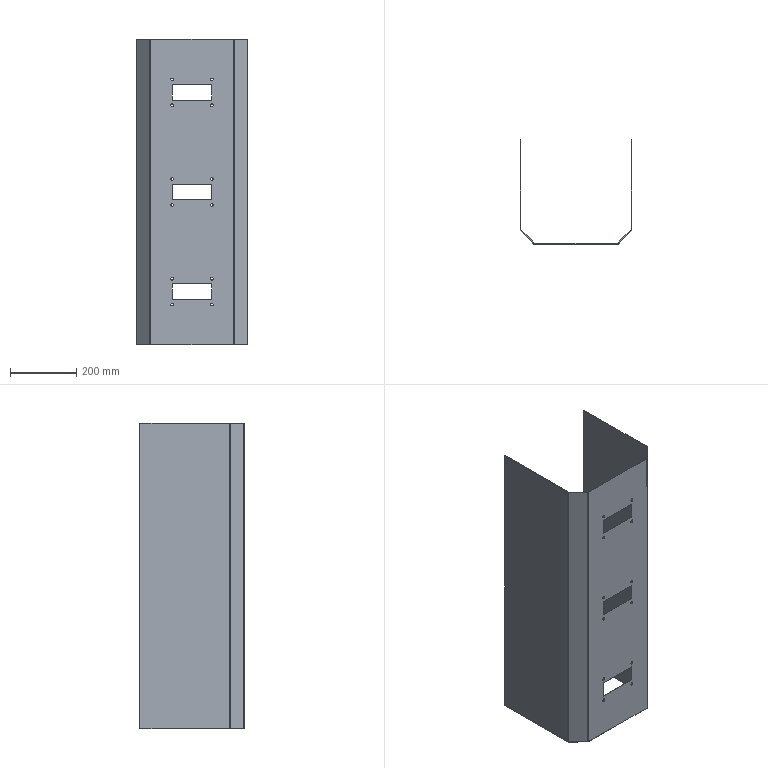Part | SolidWorks | features MirrorPattern 2, FlatPattern 1, ICE 1, SMBaseFlange 1, SheetMetal 1 | 1 solid | 74 faces | box 337 x 313.5 x 920 mm | volume 1639360 mm3 | plane 42 | cylinder 32 | commonest cylinder face diameters 8 x24 1.473 x4 5.473 x4